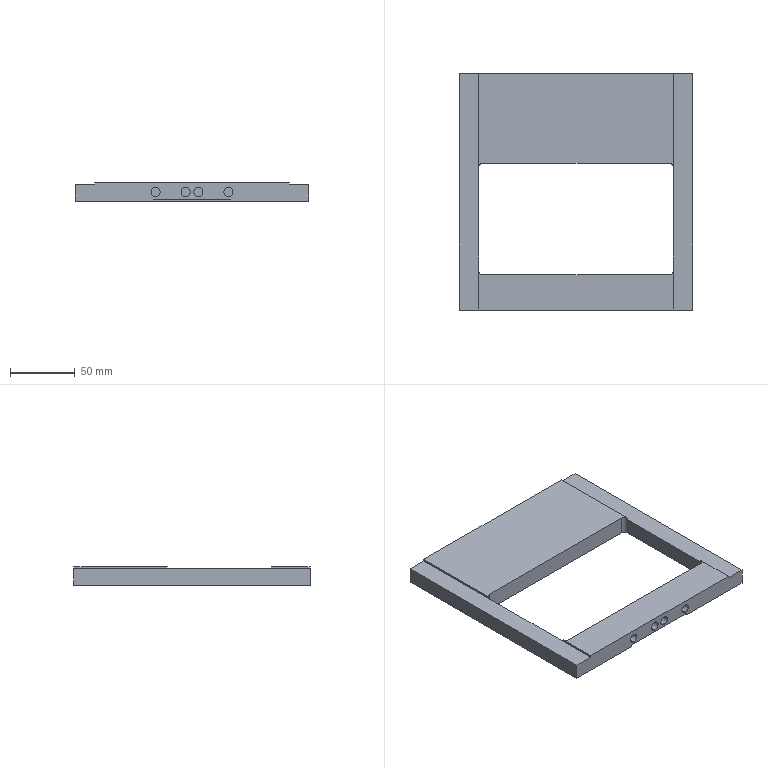Part | SolidWorks | features ICE 5, Extrusion 1, Fillet 1 | 1 solid | 47 faces | box 180 x 182 x 14 mm | volume 257706 mm3 | plane 29 | cylinder 18 | commonest cylinder face diameters 7 x8 10 x6 6 x4
STEP:
#1=CARTESIAN_POINT('',(-28.,-64.,-3.5));
#2=VERTEX_POINT('',#1);
#3=CARTESIAN_POINT('',(-28.,-64.,3.5));
#4=VERTEX_POINT('',#3);
#5=CARTESIAN_POINT('',(-28.,-64.,0.));
#6=DIRECTION('',(0.,1.,0.));
#7=DIRECTION('',(0.,0.,-1.));
#8=AXIS2_PLACEMENT_3D('',#5,#6,#7);
#9=CIRCLE('',#8,3.5);
#10=EDGE_CURVE('',#2,#4,#9,.T.);
#11=ORIENTED_EDGE('',*,*,#10,.T.);
#12=CARTESIAN_POINT('',(-28.,-91.,3.5));
#13=VERTEX_POINT('',#12);
#14=CARTESIAN_POINT('',(-28.,91.001,3.5));
#15=DIRECTION('',(0.,-1.,0.));
#16=VECTOR('',#15,1000.);
#17=LINE('',#14,#16);
#18=EDGE_CURVE('',#4,#13,#17,.T.);
#19=ORIENTED_EDGE('',*,*,#18,.T.);
#20=CARTESIAN_POINT('',(-28.,-91.,-3.5));
#21=VERTEX_POINT('',#20);
#22=CARTESIAN_POINT('',(-28.,-91.,0.));
#23=DIRECTION('',(0.,-1.,0.));
#24=DIRECTION('',(0.,0.,-1.));
#25=AXIS2_PLACEMENT_3D('',#22,#23,#24);
#26=CIRCLE('',#25,3.5);
#27=EDGE_CURVE('',#13,#21,#26,.T.);
#28=ORIENTED_EDGE('',*,*,#27,.T.);
#29=CARTESIAN_POINT('',(-28.,91.001,-3.5));
#30=DIRECTION('',(0.,-1.,0.));
#31=VECTOR('',#30,1000.);
#32=LINE('',#29,#31);
#33=EDGE_CURVE('',#2,#21,#32,.T.);
#34=ORIENTED_EDGE('',*,*,#33,.F.);
#35=EDGE_LOOP('',(#11,#19,#28,#34));
#36=FACE_OUTER_BOUND('',#35,.T.);
#37=CARTESIAN_POINT('',(-28.,91.001,0.));
#38=DIRECTION('',(0.,-1.,0.));
#39=DIRECTION('',(0.,0.,-1.));
#40=AXIS2_PLACEMENT_3D('',#37,#38,#39);
#41=CYLINDRICAL_SURFACE('',#40,3.5);
#42=ADVANCED_FACE('',(#36),#41,.F.);
#43=CARTESIAN_POINT('',(28.,-64.,-3.5));
#44=VERTEX_POINT('',#43);
#45=CARTESIAN_POINT('',(28.,-64.,3.5));
#46=VERTEX_POINT('',#45);
#47=CARTESIAN_POINT('',(28.,-64.,0.));
#48=DIRECTION('',(0.,1.,0.));
#49=DIRECTION('',(0.,0.,-1.));
#50=AXIS2_PLACEMENT_3D('',#47,#48,#49);
#51=CIRCLE('',#50,3.5);
#52=EDGE_CURVE('',#44,#46,#51,.T.);
#53=ORIENTED_EDGE('',*,*,#52,.T.);
#54=CARTESIAN_POINT('',(28.,-91.,3.5));
#55=VERTEX_POINT('',#54);
#56=CARTESIAN_POINT('',(28.,91.001,3.5));
#57=DIRECTION('',(0.,-1.,0.));
#58=VECTOR('',#57,1000.);
#59=LINE('',#56,#58);
#60=EDGE_CURVE('',#46,#55,#59,.T.);
#61=ORIENTED_EDGE('',*,*,#60,.T.);
#62=CARTESIAN_POINT('',(28.,-91.,-3.5));
#63=VERTEX_POINT('',#62);
#64=CARTESIAN_POINT('',(28.,-91.,0.));
#65=DIRECTION('',(0.,-1.,0.));
#66=DIRECTION('',(0.,0.,-1.));
#67=AXIS2_PLACEMENT_3D('',#64,#65,#66);
#68=CIRCLE('',#67,3.5);
#69=EDGE_CURVE('',#55,#63,#68,.T.);
#70=ORIENTED_EDGE('',*,*,#69,.T.);
#71=CARTESIAN_POINT('',(28.,91.001,-3.5));
#72=DIRECTION('',(0.,-1.,0.));
#73=VECTOR('',#72,1000.);
#74=LINE('',#71,#73);
#75=EDGE_CURVE('',#44,#63,#74,.T.);
#76=ORIENTED_EDGE('',*,*,#75,.F.);
#77=EDGE_LOOP('',(#53,#61,#70,#76));
#78=FACE_OUTER_BOUND('',#77,.T.);
#79=CARTESIAN_POINT('',(28.,91.001,0.));
#80=DIRECTION('',(0.,-1.,0.));
#81=DIRECTION('',(0.,0.,-1.));
#82=AXIS2_PLACEMENT_3D('',#79,#80,#81);
#83=CYLINDRICAL_SURFACE('',#82,3.5);
#84=ADVANCED_FACE('',(#78),#83,.F.);
#85=CARTESIAN_POINT('',(5.,-64.,-3.5));
#86=VERTEX_POINT('',#85);
#87=CARTESIAN_POINT('',(5.,-64.,3.5));
#88=VERTEX_POINT('',#87);
#89=CARTESIAN_POINT('',(5.,-64.,0.));
#90=DIRECTION('',(0.,1.,0.));
#91=DIRECTION('',(0.,0.,-1.));
#92=AXIS2_PLACEMENT_3D('',#89,#90,#91);
#93=CIRCLE('',#92,3.5);
#94=EDGE_CURVE('',#86,#88,#93,.T.);
#95=ORIENTED_EDGE('',*,*,#94,.T.);
#96=CARTESIAN_POINT('',(5.,-91.,3.5));
#97=VERTEX_POINT('',#96);
#98=CARTESIAN_POINT('',(5.,91.001,3.5));
#99=DIRECTION('',(0.,-1.,0.));
#100=VECTOR('',#99,1000.);
#101=LINE('',#98,#100);
#102=EDGE_CURVE('',#88,#97,#101,.T.);
#103=ORIENTED_EDGE('',*,*,#102,.T.);
#104=CARTESIAN_POINT('',(5.,-91.,-3.5));
#105=VERTEX_POINT('',#104);
#106=CARTESIAN_POINT('',(5.,-91.,0.));
#107=DIRECTION('',(0.,-1.,0.));
#108=DIRECTION('',(0.,0.,-1.));
#109=AXIS2_PLACEMENT_3D('',#106,#107,#108);
#110=CIRCLE('',#109,3.5);
#111=EDGE_CURVE('',#97,#105,#110,.T.);
#112=ORIENTED_EDGE('',*,*,#111,.T.);
#113=CARTESIAN_POINT('',(5.,91.001,-3.5));
#114=DIRECTION('',(0.,-1.,0.));
#115=VECTOR('',#114,1000.);
#116=LINE('',#113,#115);
#117=EDGE_CURVE('',#86,#105,#116,.T.);
#118=ORIENTED_EDGE('',*,*,#117,.F.);
#119=EDGE_LOOP('',(#95,#103,#112,#118));
#120=FACE_OUTER_BOUND('',#119,.T.);
#121=CARTESIAN_POINT('',(5.,91.001,0.));
#122=DIRECTION('',(0.,-1.,0.));
#123=DIRECTION('',(0.,0.,-1.));
#124=AXIS2_PLACEMENT_3D('',#121,#122,#123);
#125=CYLINDRICAL_SURFACE('',#124,3.5);
#126=ADVANCED_FACE('',(#120),#125,.F.);
#127=CARTESIAN_POINT('',(-5.,-64.,-3.5));
#128=VERTEX_POINT('',#127);
#129=CARTESIAN_POINT('',(-5.,-64.,3.5));
#130=VERTEX_POINT('',#129);
#131=CARTESIAN_POINT('',(-5.,-64.,0.));
#132=DIRECTION('',(0.,1.,0.));
#133=DIRECTION('',(0.,0.,-1.));
#134=AXIS2_PLACEMENT_3D('',#131,#132,#133);
#135=CIRCLE('',#134,3.5);
#136=EDGE_CURVE('',#128,#130,#135,.T.);
#137=ORIENTED_EDGE('',*,*,#136,.T.);
#138=CARTESIAN_POINT('',(-5.,-91.,3.5));
#139=VERTEX_POINT('',#138);
#140=CARTESIAN_POINT('',(-5.,91.001,3.5));
#141=DIRECTION('',(0.,-1.,0.));
#142=VECTOR('',#141,1000.);
#143=LINE('',#140,#142);
#144=EDGE_CURVE('',#130,#139,#143,.T.);
#145=ORIENTED_EDGE('',*,*,#144,.T.);
#146=CARTESIAN_POINT('',(-5.,-91.,-3.5));
#147=VERTEX_POINT('',#146);
#148=CARTESIAN_POINT('',(-5.,-91.,0.));
#149=DIRECTION('',(0.,-1.,0.));
#150=DIRECTION('',(0.,0.,-1.));
#151=AXIS2_PLACEMENT_3D('',#148,#149,#150);
#152=CIRCLE('',#151,3.5);
#153=EDGE_CURVE('',#139,#147,#152,.T.);
#154=ORIENTED_EDGE('',*,*,#153,.T.);
#155=CARTESIAN_POINT('',(-5.,91.001,-3.5));
#156=DIRECTION('',(0.,-1.,0.));
#157=VECTOR('',#156,1000.);
#158=LINE('',#155,#157);
#159=EDGE_CURVE('',#128,#147,#158,.T.);
#160=ORIENTED_EDGE('',*,*,#159,.F.);
#161=EDGE_LOOP('',(#137,#145,#154,#160));
#162=FACE_OUTER_BOUND('',#161,.T.);
#163=CARTESIAN_POINT('',(-5.,91.001,0.));
#164=DIRECTION('',(0.,-1.,0.));
#165=DIRECTION('',(0.,0.,-1.));
#166=AXIS2_PLACEMENT_3D('',#163,#164,#165);
#167=CYLINDRICAL_SURFACE('',#166,3.5);
#168=ADVANCED_FACE('',(#162),#167,.F.);
#169=CARTESIAN_POINT('',(-37.,-74.,-5.5));
#170=VERTEX_POINT('',#169);
#171=CARTESIAN_POINT('',(-32.,-69.,-5.5));
#172=VERTEX_POINT('',#171);
#173=CARTESIAN_POINT('',(-32.,-74.,-5.5));
#174=DIRECTION('',(0.,0.,-1.));
#175=DIRECTION('',(1.,0.,0.));
#176=AXIS2_PLACEMENT_3D('',#173,#174,#175);
#177=CIRCLE('',#176,5.);
#178=EDGE_CURVE('',#170,#172,#177,.T.);
#179=ORIENTED_EDGE('',*,*,#178,.F.);
#180=CARTESIAN_POINT('',(-37.,-74.,-7.));
#181=VERTEX_POINT('',#180);
#182=CARTESIAN_POINT('',(-37.,-74.,6.707));
#183=DIRECTION('',(0.,0.,-1.));
#184=VECTOR('',#183,1000.);
#185=LINE('',#182,#184);
#186=EDGE_CURVE('',#170,#181,#185,.T.);
#187=ORIENTED_EDGE('',*,*,#186,.T.);
#188=CARTESIAN_POINT('',(-32.,-69.,-7.));
#189=VERTEX_POINT('',#188);
#190=CARTESIAN_POINT('',(-32.,-74.,-7.));
#191=DIRECTION('',(0.,0.,-1.));
#192=DIRECTION('',(1.,0.,0.));
#193=AXIS2_PLACEMENT_3D('',#190,#191,#192);
#194=CIRCLE('',#193,5.);
#195=EDGE_CURVE('',#181,#189,#194,.T.);
#196=ORIENTED_EDGE('',*,*,#195,.T.);
#197=CARTESIAN_POINT('',(-32.,-69.,6.707));
#198=DIRECTION('',(0.,0.,-1.));
#199=VECTOR('',#198,1000.);
#200=LINE('',#197,#199);
#201=EDGE_CURVE('',#172,#189,#200,.T.);
#202=ORIENTED_EDGE('',*,*,#201,.F.);
#203=EDGE_LOOP('',(#179,#187,#196,#202));
#204=FACE_OUTER_BOUND('',#203,.T.);
#205=CARTESIAN_POINT('',(-32.,-74.,6.707));
#206=DIRECTION('',(0.,0.,-1.));
#207=DIRECTION('',(-1.,0.,0.));
#208=AXIS2_PLACEMENT_3D('',#205,#206,#207);
#209=CYLINDRICAL_SURFACE('',#208,5.);
#210=ADVANCED_FACE('',(#204),#209,.F.);
#211=CARTESIAN_POINT('',(-37.,32.,-5.5));
#212=VERTEX_POINT('',#211);
#213=CARTESIAN_POINT('',(-32.,37.,-5.5));
#214=VERTEX_POINT('',#213);
#215=CARTESIAN_POINT('',(-32.,32.,-5.5));
#216=DIRECTION('',(0.,0.,-1.));
#217=DIRECTION('',(1.,0.,0.));
#218=AXIS2_PLACEMENT_3D('',#215,#216,#217);
#219=CIRCLE('',#218,5.);
#220=EDGE_CURVE('',#212,#214,#219,.T.);
#221=ORIENTED_EDGE('',*,*,#220,.F.);
#222=CARTESIAN_POINT('',(-37.,32.,-7.));
#223=VERTEX_POINT('',#222);
#224=CARTESIAN_POINT('',(-37.,32.,6.707));
#225=DIRECTION('',(0.,0.,-1.));
#226=VECTOR('',#225,1000.);
#227=LINE('',#224,#226);
#228=EDGE_CURVE('',#212,#223,#227,.T.);
#229=ORIENTED_EDGE('',*,*,#228,.T.);
#230=CARTESIAN_POINT('',(-32.,37.,-7.));
#231=VERTEX_POINT('',#230);
#232=CARTESIAN_POINT('',(-32.,32.,-7.));
#233=DIRECTION('',(0.,0.,-1.));
#234=DIRECTION('',(-1.,0.,0.));
#235=AXIS2_PLACEMENT_3D('',#232,#233,#234);
#236=CIRCLE('',#235,5.);
#237=EDGE_CURVE('',#223,#231,#236,.T.);
#238=ORIENTED_EDGE('',*,*,#237,.T.);
#239=CARTESIAN_POINT('',(-32.,37.,6.707));
#240=DIRECTION('',(0.,0.,-1.));
#241=VECTOR('',#240,1000.);
#242=LINE('',#239,#241);
#243=EDGE_CURVE('',#214,#231,#242,.T.);
#244=ORIENTED_EDGE('',*,*,#243,.F.);
#245=EDGE_LOOP('',(#221,#229,#238,#244));
#246=FACE_OUTER_BOUND('',#245,.T.);
#247=CARTESIAN_POINT('',(-32.,32.,6.707));
#248=DIRECTION('',(0.,0.,-1.));
#249=DIRECTION('',(-1.,0.,0.));
#250=AXIS2_PLACEMENT_3D('',#247,#248,#249);
#251=CYLINDRICAL_SURFACE('',#250,5.);
#252=ADVANCED_FACE('',(#246),#251,.F.);
#253=CARTESIAN_POINT('',(-90.,91.,5.5));
#254=VERTEX_POINT('',#253);
#255=CARTESIAN_POINT('',(-90.,-91.,5.5));
#256=VERTEX_POINT('',#255);
#257=CARTESIAN_POINT('',(-90.,91.,5.5));
#258=DIRECTION('',(0.,-1.,0.));
#259=VECTOR('',#258,1000.);
#260=LINE('',#257,#259);
#261=EDGE_CURVE('',#254,#256,#260,.T.);
#262=ORIENTED_EDGE('',*,*,#261,.F.);
#263=CARTESIAN_POINT('',(-90.,91.,-7.));
#264=VERTEX_POINT('',#263);
#265=CARTESIAN_POINT('',(-90.,91.,7.));
#266=DIRECTION('',(0.,0.,-1.));
#267=VECTOR('',#266,1000.);
#268=LINE('',#265,#267);
#269=EDGE_CURVE('',#254,#264,#268,.T.);
#270=ORIENTED_EDGE('',*,*,#269,.T.);
#271=CARTESIAN_POINT('',(-90.,-91.,-7.));
#272=VERTEX_POINT('',#271);
#273=CARTESIAN_POINT('',(-90.,-91.,-7.));
#274=DIRECTION('',(0.,-1.,0.));
#275=VECTOR('',#274,1000.);
#276=LINE('',#273,#275);
#277=EDGE_CURVE('',#264,#272,#276,.T.);
#278=ORIENTED_EDGE('',*,*,#277,.T.);
#279=CARTESIAN_POINT('',(-90.,-91.,7.));
#280=DIRECTION('',(0.,0.,-1.));
#281=VECTOR('',#280,1000.);
#282=LINE('',#279,#281);
#283=EDGE_CURVE('',#256,#272,#282,.T.);
#284=ORIENTED_EDGE('',*,*,#283,.F.);
#285=EDGE_LOOP('',(#262,#270,#278,#284));
#286=FACE_OUTER_BOUND('',#285,.T.);
#287=CARTESIAN_POINT('',(-90.,-91.,7.));
#288=DIRECTION('',(1.,0.,0.));
#289=DIRECTION('',(0.,0.,-1.));
#290=AXIS2_PLACEMENT_3D('',#287,#288,#289);
#291=PLANE('',#290);
#292=ADVANCED_FACE('',(#286),#291,.F.);
#293=CARTESIAN_POINT('',(75.,91.,7.));
#294=VERTEX_POINT('',#293);
#295=CARTESIAN_POINT('',(-75.,91.,7.));
#296=VERTEX_POINT('',#295);
#297=CARTESIAN_POINT('',(-90.,91.,7.));
#298=DIRECTION('',(-1.,0.,0.));
#299=VECTOR('',#298,1000.);
#300=LINE('',#297,#299);
#301=EDGE_CURVE('',#294,#296,#300,.T.);
#302=ORIENTED_EDGE('',*,*,#301,.T.);
#303=CARTESIAN_POINT('',(-75.,19.,7.));
#304=VERTEX_POINT('',#303);
#305=CARTESIAN_POINT('',(-75.,91.,7.));
#306=DIRECTION('',(0.,1.,0.));
#307=VECTOR('',#306,1000.);
#308=LINE('',#305,#307);
#309=EDGE_CURVE('',#304,#296,#308,.T.);
#310=ORIENTED_EDGE('',*,*,#309,.F.);
#311=CARTESIAN_POINT('',(-72.,22.,7.));
#312=VERTEX_POINT('',#311);
#313=CARTESIAN_POINT('',(-72.,19.,7.));
#314=DIRECTION('',(0.,0.,-1.));
#315=DIRECTION('',(-1.,0.,0.));
#316=AXIS2_PLACEMENT_3D('',#313,#314,#315);
#317=CIRCLE('',#316,3.);
#318=EDGE_CURVE('',#304,#312,#317,.T.);
#319=ORIENTED_EDGE('',*,*,#318,.T.);
#320=CARTESIAN_POINT('',(72.,22.,7.));
#321=VERTEX_POINT('',#320);
#322=CARTESIAN_POINT('',(75.,22.,7.));
#323=DIRECTION('',(-1.,0.,0.));
#324=VECTOR('',#323,1000.);
#325=LINE('',#322,#324);
#326=EDGE_CURVE('',#321,#312,#325,.T.);
#327=ORIENTED_EDGE('',*,*,#326,.F.);
#328=CARTESIAN_POINT('',(75.,19.,7.));
#329=VERTEX_POINT('',#328);
#330=CARTESIAN_POINT('',(72.,19.,7.));
#331=DIRECTION('',(0.,0.,-1.));
#332=DIRECTION('',(-1.,0.,0.));
#333=AXIS2_PLACEMENT_3D('',#330,#331,#332);
#334=CIRCLE('',#333,3.);
#335=EDGE_CURVE('',#321,#329,#334,.T.);
#336=ORIENTED_EDGE('',*,*,#335,.T.);
#337=CARTESIAN_POINT('',(75.,91.,7.));
#338=DIRECTION('',(0.,-1.,0.));
#339=VECTOR('',#338,1000.);
#340=LINE('',#337,#339);
#341=EDGE_CURVE('',#294,#329,#340,.T.);
#342=ORIENTED_EDGE('',*,*,#341,.F.);
#343=EDGE_LOOP('',(#302,#310,#319,#327,#336,#342));
#344=FACE_OUTER_BOUND('',#343,.T.);
#345=CARTESIAN_POINT('',(0.,0.,7.));
#346=DIRECTION('',(0.,0.,-1.));
#347=DIRECTION('',(-1.,0.,0.));
#348=AXIS2_PLACEMENT_3D('',#345,#346,#347);
#349=PLANE('',#348);
#350=ADVANCED_FACE('',(#344),#349,.F.);
#351=CARTESIAN_POINT('',(-75.,-61.,5.5));
#352=VERTEX_POINT('',#351);
#353=CARTESIAN_POINT('',(-75.,19.,5.5));
#354=VERTEX_POINT('',#353);
#355=CARTESIAN_POINT('',(-75.,91.,5.5));
#356=DIRECTION('',(0.,1.,0.));
#357=VECTOR('',#356,1000.);
#358=LINE('',#355,#357);
#359=EDGE_CURVE('',#352,#354,#358,.T.);
#360=ORIENTED_EDGE('',*,*,#359,.F.);
#361=CARTESIAN_POINT('',(-75.,-61.,-7.));
#362=VERTEX_POINT('',#361);
#363=CARTESIAN_POINT('',(-75.,-61.,-7.));
#364=DIRECTION('',(0.,0.,-1.));
#365=VECTOR('',#364,1000.);
#366=LINE('',#363,#365);
#367=EDGE_CURVE('',#352,#362,#366,.T.);
#368=ORIENTED_EDGE('',*,*,#367,.T.);
#369=CARTESIAN_POINT('',(-75.,19.,-7.));
#370=VERTEX_POINT('',#369);
#371=CARTESIAN_POINT('',(-75.,-64.,-7.));
#372=DIRECTION('',(0.,1.,0.));
#373=VECTOR('',#372,1000.);
#374=LINE('',#371,#373);
#375=EDGE_CURVE('',#362,#370,#374,.T.);
#376=ORIENTED_EDGE('',*,*,#375,.T.);
#377=CARTESIAN_POINT('',(-75.,19.,7.));
#378=DIRECTION('',(0.,0.,1.));
#379=VECTOR('',#378,1000.);
#380=LINE('',#377,#379);
#381=EDGE_CURVE('',#370,#354,#380,.T.);
#382=ORIENTED_EDGE('',*,*,#381,.T.);
#383=EDGE_LOOP('',(#360,#368,#376,#382));
#384=FACE_OUTER_BOUND('',#383,.T.);
#385=CARTESIAN_POINT('',(-75.,-64.,7.001));
#386=DIRECTION('',(-1.,0.,0.));
#387=DIRECTION('',(0.,0.,1.));
#388=AXIS2_PLACEMENT_3D('',#385,#386,#387);
#389=PLANE('',#388);
#390=ADVANCED_FACE('',(#384),#389,.F.);
#391=CARTESIAN_POINT('',(90.,91.,5.5));
#392=VERTEX_POINT('',#391);
#393=CARTESIAN_POINT('',(90.,91.,-7.));
#394=VERTEX_POINT('',#393);
#395=CARTESIAN_POINT('',(90.,91.,7.));
#396=DIRECTION('',(0.,0.,-1.));
#397=VECTOR('',#396,1000.);
#398=LINE('',#395,#397);
#399=EDGE_CURVE('',#392,#394,#398,.T.);
#400=ORIENTED_EDGE('',*,*,#399,.F.);
#401=CARTESIAN_POINT('',(90.,-91.,5.5));
#402=VERTEX_POINT('',#401);
#403=CARTESIAN_POINT('',(90.,91.,5.5));
#404=DIRECTION('',(0.,1.,0.));
#405=VECTOR('',#404,1000.);
#406=LINE('',#403,#405);
#407=EDGE_CURVE('',#402,#392,#406,.T.);
#408=ORIENTED_EDGE('',*,*,#407,.F.);
#409=CARTESIAN_POINT('',(90.,-91.,-7.));
#410=VERTEX_POINT('',#409);
#411=CARTESIAN_POINT('',(90.,-91.,7.));
#412=DIRECTION('',(0.,0.,-1.));
#413=VECTOR('',#412,1000.);
#414=LINE('',#411,#413);
#415=EDGE_CURVE('',#402,#410,#414,.T.);
#416=ORIENTED_EDGE('',*,*,#415,.T.);
#417=CARTESIAN_POINT('',(90.,-91.,-7.));
#418=DIRECTION('',(0.,1.,0.));
#419=VECTOR('',#418,1000.);
#420=LINE('',#417,#419);
#421=EDGE_CURVE('',#410,#394,#420,.T.);
#422=ORIENTED_EDGE('',*,*,#421,.T.);
#423=EDGE_LOOP('',(#400,#408,#416,#422));
#424=FACE_OUTER_BOUND('',#423,.T.);
#425=CARTESIAN_POINT('',(90.,-91.,7.));
#426=DIRECTION('',(-1.,0.,0.));
#427=DIRECTION('',(0.,0.,1.));
#428=AXIS2_PLACEMENT_3D('',#425,#426,#427);
#429=PLANE('',#428);
#430=ADVANCED_FACE('',(#424),#429,.F.);
#431=CARTESIAN_POINT('',(-75.,91.,5.5));
#432=VERTEX_POINT('',#431);
#433=CARTESIAN_POINT('',(-90.,91.,5.5));
#434=DIRECTION('',(-1.,0.,0.));
#435=VECTOR('',#434,1000.);
#436=LINE('',#433,#435);
#437=EDGE_CURVE('',#432,#254,#436,.T.);
#438=ORIENTED_EDGE('',*,*,#437,.F.);
#439=CARTESIAN_POINT('',(-75.,91.,5.5));
#440=DIRECTION('',(0.,0.,1.));
#441=VECTOR('',#440,1000.);
#442=LINE('',#439,#441);
#443=EDGE_CURVE('',#432,#296,#442,.T.);
#444=ORIENTED_EDGE('',*,*,#443,.T.);
#445=ORIENTED_EDGE('',*,*,#301,.F.);
#446=CARTESIAN_POINT('',(75.,91.,5.5));
#447=VERTEX_POINT('',#446);
#448=CARTESIAN_POINT('',(75.,91.,5.5));
#449=DIRECTION('',(0.,0.,1.));
#450=VECTOR('',#449,1000.);
#451=LINE('',#448,#450);
#452=EDGE_CURVE('',#447,#294,#451,.T.);
#453=ORIENTED_EDGE('',*,*,#452,.F.);
#454=CARTESIAN_POINT('',(90.,91.,5.5));
#455=DIRECTION('',(-1.,0.,0.));
#456=VECTOR('',#455,1000.);
#457=LINE('',#454,#456);
#458=EDGE_CURVE('',#392,#447,#457,.T.);
#459=ORIENTED_EDGE('',*,*,#458,.F.);
#460=ORIENTED_EDGE('',*,*,#399,.T.);
#461=CARTESIAN_POINT('',(30.,91.,-7.));
#462=VERTEX_POINT('',#461);
#463=CARTESIAN_POINT('',(-90.,91.,-7.));
#464=DIRECTION('',(-1.,0.,0.));
#465=VECTOR('',#464,1000.);
#466=LINE('',#463,#465);
#467=EDGE_CURVE('',#394,#462,#466,.T.);
#468=ORIENTED_EDGE('',*,*,#467,.T.);
#469=CARTESIAN_POINT('',(30.,91.,-5.5));
#470=VERTEX_POINT('',#469);
#471=CARTESIAN_POINT('',(30.,91.,-5.5));
#472=DIRECTION('',(0.,0.,-1.));
#473=VECTOR('',#472,1000.);
#474=LINE('',#471,#473);
#475=EDGE_CURVE('',#470,#462,#474,.T.);
#476=ORIENTED_EDGE('',*,*,#475,.F.);
#477=CARTESIAN_POINT('',(-30.,91.,-5.5));
#478=VERTEX_POINT('',#477);
#479=CARTESIAN_POINT('',(30.,91.,-5.5));
#480=DIRECTION('',(1.,0.,0.));
#481=VECTOR('',#480,1000.);
#482=LINE('',#479,#481);
#483=EDGE_CURVE('',#478,#470,#482,.T.);
#484=ORIENTED_EDGE('',*,*,#483,.F.);
#485=CARTESIAN_POINT('',(-30.,91.,-7.));
#486=VERTEX_POINT('',#485);
#487=CARTESIAN_POINT('',(-30.,91.,-5.5));
#488=DIRECTION('',(0.,0.,-1.));
#489=VECTOR('',#488,1000.);
#490=LINE('',#487,#489);
#491=EDGE_CURVE('',#478,#486,#490,.T.);
#492=ORIENTED_EDGE('',*,*,#491,.T.);
#493=CARTESIAN_POINT('',(-90.,91.,-7.));
#494=DIRECTION('',(-1.,0.,0.));
#495=VECTOR('',#494,1000.);
#496=LINE('',#493,#495);
#497=EDGE_CURVE('',#486,#264,#496,.T.);
#498=ORIENTED_EDGE('',*,*,#497,.T.);
#499=ORIENTED_EDGE('',*,*,#269,.F.);
#500=EDGE_LOOP('',(#438,#444,#445,#453,#459,#460,#468,#476,#484,#492,#498,#499));
#501=FACE_OUTER_BOUND('',#500,.T.);
#502=CARTESIAN_POINT('',(-90.,91.,7.));
#503=DIRECTION('',(0.,-1.,0.));
#504=DIRECTION('',(0.,0.,-1.));
#505=AXIS2_PLACEMENT_3D('',#502,#503,#504);
#506=PLANE('',#505);
#507=ADVANCED_FACE('',(#501),#506,.F.);
#508=CARTESIAN_POINT('',(-28.,-91.,0.));
#509=DIRECTION('',(0.,-1.,0.));
#510=DIRECTION('',(0.,0.,-1.));
#511=AXIS2_PLACEMENT_3D('',#508,#509,#510);
#512=CIRCLE('',#511,3.5);
#513=EDGE_CURVE('',#21,#13,#512,.T.);
#514=ORIENTED_EDGE('',*,*,#513,.F.);
#515=ORIENTED_EDGE('',*,*,#27,.F.);
#516=EDGE_LOOP('',(#514,#515));
#517=FACE_BOUND('',#516,.T.);
#518=CARTESIAN_POINT('',(28.,-91.,0.));
#519=DIRECTION('',(0.,-1.,0.));
#520=DIRECTION('',(0.,0.,-1.));
#521=AXIS2_PLACEMENT_3D('',#518,#519,#520);
#522=CIRCLE('',#521,3.5);
#523=EDGE_CURVE('',#63,#55,#522,.T.);
#524=ORIENTED_EDGE('',*,*,#523,.F.);
#525=ORIENTED_EDGE('',*,*,#69,.F.);
#526=EDGE_LOOP('',(#524,#525));
#527=FACE_BOUND('',#526,.T.);
#528=CARTESIAN_POINT('',(5.,-91.,0.));
#529=DIRECTION('',(0.,-1.,0.));
#530=DIRECTION('',(0.,0.,-1.));
#531=AXIS2_PLACEMENT_3D('',#528,#529,#530);
#532=CIRCLE('',#531,3.5);
#533=EDGE_CURVE('',#105,#97,#532,.T.);
#534=ORIENTED_EDGE('',*,*,#533,.F.);
#535=ORIENTED_EDGE('',*,*,#111,.F.);
#536=EDGE_LOOP('',(#534,#535));
#537=FACE_BOUND('',#536,.T.);
#538=CARTESIAN_POINT('',(-5.,-91.,0.));
#539=DIRECTION('',(0.,-1.,0.));
#540=DIRECTION('',(0.,0.,-1.));
#541=AXIS2_PLACEMENT_3D('',#538,#539,#540);
#542=CIRCLE('',#541,3.5);
#543=EDGE_CURVE('',#147,#139,#542,.T.);
#544=ORIENTED_EDGE('',*,*,#543,.F.);
#545=ORIENTED_EDGE('',*,*,#153,.F.);
#546=EDGE_LOOP('',(#544,#545));
#547=FACE_BOUND('',#546,.T.);
#548=CARTESIAN_POINT('',(-75.,-91.,7.));
#549=VERTEX_POINT('',#548);
#550=CARTESIAN_POINT('',(75.,-91.,7.));
#551=VERTEX_POINT('',#550);
#552=CARTESIAN_POINT('',(-90.,-91.,7.));
#553=DIRECTION('',(1.,0.,0.));
#554=VECTOR('',#553,1000.);
#555=LINE('',#552,#554);
#556=EDGE_CURVE('',#549,#551,#555,.T.);
#557=ORIENTED_EDGE('',*,*,#556,.F.);
#558=CARTESIAN_POINT('',(-75.,-91.,5.5));
#559=VERTEX_POINT('',#558);
#560=CARTESIAN_POINT('',(-75.,-91.,5.5));
#561=DIRECTION('',(0.,0.,1.));
#562=VECTOR('',#561,1000.);
#563=LINE('',#560,#562);
#564=EDGE_CURVE('',#559,#549,#563,.T.);
#565=ORIENTED_EDGE('',*,*,#564,.F.);
#566=CARTESIAN_POINT('',(-90.,-91.,5.5));
#567=DIRECTION('',(1.,0.,0.));
#568=VECTOR('',#567,1000.);
#569=LINE('',#566,#568);
#570=EDGE_CURVE('',#256,#559,#569,.T.);
#571=ORIENTED_EDGE('',*,*,#570,.F.);
#572=ORIENTED_EDGE('',*,*,#283,.T.);
#573=CARTESIAN_POINT('',(-30.,-91.,-7.));
#574=VERTEX_POINT('',#573);
#575=CARTESIAN_POINT('',(-90.,-91.,-7.));
#576=DIRECTION('',(1.,0.,0.));
#577=VECTOR('',#576,1000.);
#578=LINE('',#575,#577);
#579=EDGE_CURVE('',#272,#574,#578,.T.);
#580=ORIENTED_EDGE('',*,*,#579,.T.);
#581=CARTESIAN_POINT('',(-30.,-91.,-5.5));
#582=VERTEX_POINT('',#581);
#583=CARTESIAN_POINT('',(-30.,-91.,-5.5));
#584=DIRECTION('',(0.,0.,-1.));
#585=VECTOR('',#584,1000.);
#586=LINE('',#583,#585);
#587=EDGE_CURVE('',#582,#574,#586,.T.);
#588=ORIENTED_EDGE('',*,*,#587,.F.);
#589=CARTESIAN_POINT('',(30.,-91.,-5.5));
#590=VERTEX_POINT('',#589);
#591=CARTESIAN_POINT('',(30.,-91.,-5.5));
#592=DIRECTION('',(-1.,0.,0.));
#593=VECTOR('',#592,1000.);
#594=LINE('',#591,#593);
#595=EDGE_CURVE('',#590,#582,#594,.T.);
#596=ORIENTED_EDGE('',*,*,#595,.F.);
#597=CARTESIAN_POINT('',(30.,-91.,-7.));
#598=VERTEX_POINT('',#597);
#599=CARTESIAN_POINT('',(30.,-91.,-5.5));
#600=DIRECTION('',(0.,0.,-1.));
#601=VECTOR('',#600,1000.);
#602=LINE('',#599,#601);
#603=EDGE_CURVE('',#590,#598,#602,.T.);
#604=ORIENTED_EDGE('',*,*,#603,.T.);
#605=CARTESIAN_POINT('',(-90.,-91.,-7.));
#606=DIRECTION('',(1.,0.,0.));
#607=VECTOR('',#606,1000.);
#608=LINE('',#605,#607);
#609=EDGE_CURVE('',#598,#410,#608,.T.);
#610=ORIENTED_EDGE('',*,*,#609,.T.);
#611=ORIENTED_EDGE('',*,*,#415,.F.);
#612=CARTESIAN_POINT('',(75.,-91.,5.5));
#613=VERTEX_POINT('',#612);
#614=CARTESIAN_POINT('',(90.,-91.,5.5));
#615=DIRECTION('',(1.,0.,0.));
#616=VECTOR('',#615,1000.);
#617=LINE('',#614,#616);
#618=EDGE_CURVE('',#613,#402,#617,.T.);
#619=ORIENTED_EDGE('',*,*,#618,.F.);
#620=CARTESIAN_POINT('',(75.,-91.,5.5));
#621=DIRECTION('',(0.,0.,1.));
#622=VECTOR('',#621,1000.);
#623=LINE('',#620,#622);
#624=EDGE_CURVE('',#613,#551,#623,.T.);
#625=ORIENTED_EDGE('',*,*,#624,.T.);
#626=EDGE_LOOP('',(#557,#565,#571,#572,#580,#588,#596,#604,#610,#611,#619,#625));
#627=FACE_OUTER_BOUND('',#626,.T.);
#628=CARTESIAN_POINT('',(-90.,-91.,7.));
#629=DIRECTION('',(0.,1.,0.));
#630=DIRECTION('',(0.,0.,1.));
#631=AXIS2_PLACEMENT_3D('',#628,#629,#630);
#632=PLANE('',#631);
#633=ADVANCED_FACE('',(#517,#527,#537,#547,#627),#632,.F.);
#634=CARTESIAN_POINT('',(-72.,-64.,7.));
#635=VERTEX_POINT('',#634);
#636=CARTESIAN_POINT('',(-75.,-61.,7.));
#637=VERTEX_POINT('',#636);
#638=CARTESIAN_POINT('',(-72.,-61.,7.));
#639=DIRECTION('',(0.,0.,-1.));
#640=DIRECTION('',(-1.,0.,0.));
#641=AXIS2_PLACEMENT_3D('',#638,#639,#640);
#642=CIRCLE('',#641,3.);
#643=EDGE_CURVE('',#635,#637,#642,.T.);
#644=ORIENTED_EDGE('',*,*,#643,.T.);
#645=CARTESIAN_POINT('',(-75.,91.,7.));
#646=DIRECTION('',(0.,1.,0.));
#647=VECTOR('',#646,1000.);
#648=LINE('',#645,#647);
#649=EDGE_CURVE('',#549,#637,#648,.T.);
#650=ORIENTED_EDGE('',*,*,#649,.F.);
#651=ORIENTED_EDGE('',*,*,#556,.T.);
#652=CARTESIAN_POINT('',(75.,-61.,7.));
#653=VERTEX_POINT('',#652);
#654=CARTESIAN_POINT('',(75.,91.,7.));
#655=DIRECTION('',(0.,-1.,0.));
#656=VECTOR('',#655,1000.);
#657=LINE('',#654,#656);
#658=EDGE_CURVE('',#653,#551,#657,.T.);
#659=ORIENTED_EDGE('',*,*,#658,.F.);
#660=CARTESIAN_POINT('',(72.,-64.,7.));
#661=VERTEX_POINT('',#660);
#662=CARTESIAN_POINT('',(72.,-61.,7.));
#663=DIRECTION('',(0.,0.,-1.));
#664=DIRECTION('',(-1.,0.,0.));
#665=AXIS2_PLACEMENT_3D('',#662,#663,#664);
#666=CIRCLE('',#665,3.);
#667=EDGE_CURVE('',#653,#661,#666,.T.);
#668=ORIENTED_EDGE('',*,*,#667,.T.);
#669=CARTESIAN_POINT('',(75.,-64.,7.));
#670=DIRECTION('',(1.,0.,0.));
#671=VECTOR('',#670,1000.);
#672=LINE('',#669,#671);
#673=EDGE_CURVE('',#635,#661,#672,.T.);
#674=ORIENTED_EDGE('',*,*,#673,.F.);
#675=EDGE_LOOP('',(#644,#650,#651,#659,#668,#674));
#676=FACE_OUTER_BOUND('',#675,.T.);
#677=CARTESIAN_POINT('',(0.,0.,7.));
#678=DIRECTION('',(0.,0.,-1.));
#679=DIRECTION('',(-1.,0.,0.));
#680=AXIS2_PLACEMENT_3D('',#677,#678,#679);
#681=PLANE('',#680);
#682=ADVANCED_FACE('',(#676),#681,.F.);
#683=ORIENTED_EDGE('',*,*,#375,.F.);
#684=CARTESIAN_POINT('',(-72.,-64.,-7.));
#685=VERTEX_POINT('',#684);
#686=CARTESIAN_POINT('',(-72.,-61.,-7.));
#687=DIRECTION('',(0.,0.,1.));
#688=DIRECTION('',(-1.,0.,0.));
#689=AXIS2_PLACEMENT_3D('',#686,#687,#688);
#690=CIRCLE('',#689,3.);
#691=EDGE_CURVE('',#362,#685,#690,.T.);
#692=ORIENTED_EDGE('',*,*,#691,.T.);
#693=CARTESIAN_POINT('',(72.,-64.,-7.));
#694=VERTEX_POINT('',#693);
#695=CARTESIAN_POINT('',(75.,-64.,-7.));
#696=DIRECTION('',(-1.,0.,0.));
#697=VECTOR('',#696,1000.);
#698=LINE('',#695,#697);
#699=EDGE_CURVE('',#694,#685,#698,.T.);
#700=ORIENTED_EDGE('',*,*,#699,.F.);
#701=CARTESIAN_POINT('',(75.,-61.,-7.));
#702=VERTEX_POINT('',#701);
#703=CARTESIAN_POINT('',(72.,-61.,-7.));
#704=DIRECTION('',(0.,0.,1.));
#705=DIRECTION('',(-1.,0.,0.));
#706=AXIS2_PLACEMENT_3D('',#703,#704,#705);
#707=CIRCLE('',#706,3.);
#708=EDGE_CURVE('',#694,#702,#707,.T.);
#709=ORIENTED_EDGE('',*,*,#708,.T.);
#710=CARTESIAN_POINT('',(75.,19.,-7.));
#711=VERTEX_POINT('',#710);
#712=CARTESIAN_POINT('',(75.,-64.,-7.));
#713=DIRECTION('',(0.,-1.,0.));
#714=VECTOR('',#713,1000.);
#715=LINE('',#712,#714);
#716=EDGE_CURVE('',#711,#702,#715,.T.);
#717=ORIENTED_EDGE('',*,*,#716,.F.);
#718=CARTESIAN_POINT('',(72.,22.,-7.));
#719=VERTEX_POINT('',#718);
#720=CARTESIAN_POINT('',(72.,19.,-7.));
#721=DIRECTION('',(0.,0.,1.));
#722=DIRECTION('',(-1.,0.,0.));
#723=AXIS2_PLACEMENT_3D('',#720,#721,#722);
#724=CIRCLE('',#723,3.);
#725=EDGE_CURVE('',#711,#719,#724,.T.);
#726=ORIENTED_EDGE('',*,*,#725,.T.);
#727=CARTESIAN_POINT('',(-72.,22.,-7.));
#728=VERTEX_POINT('',#727);
#729=CARTESIAN_POINT('',(75.,22.,-7.));
#730=DIRECTION('',(1.,0.,0.));
#731=VECTOR('',#730,1000.);
#732=LINE('',#729,#731);
#733=EDGE_CURVE('',#728,#719,#732,.T.);
#734=ORIENTED_EDGE('',*,*,#733,.F.);
#735=CARTESIAN_POINT('',(-72.,19.,-7.));
#736=DIRECTION('',(0.,0.,1.));
#737=DIRECTION('',(-1.,0.,0.));
#738=AXIS2_PLACEMENT_3D('',#735,#736,#737);
#739=CIRCLE('',#738,3.);
#740=EDGE_CURVE('',#728,#370,#739,.T.);
#741=ORIENTED_EDGE('',*,*,#740,.T.);
#742=EDGE_LOOP('',(#683,#692,#700,#709,#717,#726,#734,#741));
#743=FACE_BOUND('',#742,.T.);
#744=CARTESIAN_POINT('',(32.,27.,-7.));
#745=VERTEX_POINT('',#744);
#746=CARTESIAN_POINT('',(-32.,27.,-7.));
#747=VERTEX_POINT('',#746);
#748=CARTESIAN_POINT('',(30.,27.,-7.));
#749=DIRECTION('',(-1.,0.,0.));
#750=VECTOR('',#749,1000.);
#751=LINE('',#748,#750);
#752=EDGE_CURVE('',#745,#747,#751,.T.);
#753=ORIENTED_EDGE('',*,*,#752,.F.);
#754=CARTESIAN_POINT('',(32.,37.,-7.));
#755=VERTEX_POINT('',#754);
#756=CARTESIAN_POINT('',(32.,32.,-7.));
#757=DIRECTION('',(0.,0.,-1.));
#758=DIRECTION('',(1.,0.,0.));
#759=AXIS2_PLACEMENT_3D('',#756,#757,#758);
#760=CIRCLE('',#759,5.);
#761=EDGE_CURVE('',#755,#745,#760,.T.);
#762=ORIENTED_EDGE('',*,*,#761,.F.);
#763=CARTESIAN_POINT('',(30.,37.,-7.));
#764=VERTEX_POINT('',#763);
#765=CARTESIAN_POINT('',(32.,37.,-7.));
#766=DIRECTION('',(1.,0.,0.));
#767=VECTOR('',#766,1000.);
#768=LINE('',#765,#767);
#769=EDGE_CURVE('',#764,#755,#768,.T.);
#770=ORIENTED_EDGE('',*,*,#769,.F.);
#771=CARTESIAN_POINT('',(30.,27.,-7.));
#772=DIRECTION('',(0.,-1.,0.));
#773=VECTOR('',#772,1000.);
#774=LINE('',#771,#773);
#775=EDGE_CURVE('',#462,#764,#774,.T.);
#776=ORIENTED_EDGE('',*,*,#775,.F.);
#777=ORIENTED_EDGE('',*,*,#467,.F.);
#778=ORIENTED_EDGE('',*,*,#421,.F.);
#779=ORIENTED_EDGE('',*,*,#609,.F.);
#780=CARTESIAN_POINT('',(30.,-79.,-7.));
#781=VERTEX_POINT('',#780);
#782=CARTESIAN_POINT('',(30.,-91.,-7.));
#783=DIRECTION('',(0.,-1.,0.));
#784=VECTOR('',#783,1000.);
#785=LINE('',#782,#784);
#786=EDGE_CURVE('',#781,#598,#785,.T.);
#787=ORIENTED_EDGE('',*,*,#786,.F.);
#788=CARTESIAN_POINT('',(32.,-79.,-7.));
#789=VERTEX_POINT('',#788);
#790=CARTESIAN_POINT('',(32.,-79.,-7.));
#791=DIRECTION('',(-1.,0.,0.));
#792=VECTOR('',#791,1000.);
#793=LINE('',#790,#792);
#794=EDGE_CURVE('',#789,#781,#793,.T.);
#795=ORIENTED_EDGE('',*,*,#794,.F.);
#796=CARTESIAN_POINT('',(32.,-69.,-7.));
#797=VERTEX_POINT('',#796);
#798=CARTESIAN_POINT('',(32.,-74.,-7.));
#799=DIRECTION('',(0.,0.,-1.));
#800=DIRECTION('',(-1.,0.,0.));
#801=AXIS2_PLACEMENT_3D('',#798,#799,#800);
#802=CIRCLE('',#801,5.);
#803=EDGE_CURVE('',#797,#789,#802,.T.);
#804=ORIENTED_EDGE('',*,*,#803,.F.);
#805=CARTESIAN_POINT('',(30.,-69.,-7.));
#806=DIRECTION('',(1.,0.,0.));
#807=VECTOR('',#806,1000.);
#808=LINE('',#805,#807);
#809=EDGE_CURVE('',#189,#797,#808,.T.);
#810=ORIENTED_EDGE('',*,*,#809,.F.);
#811=ORIENTED_EDGE('',*,*,#195,.F.);
#812=CARTESIAN_POINT('',(-32.,-79.,-7.));
#813=VERTEX_POINT('',#812);
#814=CARTESIAN_POINT('',(-32.,-74.,-7.));
#815=DIRECTION('',(0.,0.,-1.));
#816=DIRECTION('',(1.,0.,0.));
#817=AXIS2_PLACEMENT_3D('',#814,#815,#816);
#818=CIRCLE('',#817,5.);
#819=EDGE_CURVE('',#813,#181,#818,.T.);
#820=ORIENTED_EDGE('',*,*,#819,.F.);
#821=CARTESIAN_POINT('',(-30.,-79.,-7.));
#822=VERTEX_POINT('',#821);
#823=CARTESIAN_POINT('',(-32.,-79.,-7.));
#824=DIRECTION('',(-1.,0.,0.));
#825=VECTOR('',#824,1000.);
#826=LINE('',#823,#825);
#827=EDGE_CURVE('',#822,#813,#826,.T.);
#828=ORIENTED_EDGE('',*,*,#827,.F.);
#829=CARTESIAN_POINT('',(-30.,-91.,-7.));
#830=DIRECTION('',(0.,1.,0.));
#831=VECTOR('',#830,1000.);
#832=LINE('',#829,#831);
#833=EDGE_CURVE('',#574,#822,#832,.T.);
#834=ORIENTED_EDGE('',*,*,#833,.F.);
#835=ORIENTED_EDGE('',*,*,#579,.F.);
#836=ORIENTED_EDGE('',*,*,#277,.F.);
#837=ORIENTED_EDGE('',*,*,#497,.F.);
#838=CARTESIAN_POINT('',(-30.,37.,-7.));
#839=VERTEX_POINT('',#838);
#840=CARTESIAN_POINT('',(-30.,27.,-7.));
#841=DIRECTION('',(0.,1.,0.));
#842=VECTOR('',#841,1000.);
#843=LINE('',#840,#842);
#844=EDGE_CURVE('',#839,#486,#843,.T.);
#845=ORIENTED_EDGE('',*,*,#844,.F.);
#846=CARTESIAN_POINT('',(-32.,37.,-7.));
#847=DIRECTION('',(1.,0.,0.));
#848=VECTOR('',#847,1000.);
#849=LINE('',#846,#848);
#850=EDGE_CURVE('',#231,#839,#849,.T.);
#851=ORIENTED_EDGE('',*,*,#850,.F.);
#852=ORIENTED_EDGE('',*,*,#237,.F.);
#853=CARTESIAN_POINT('',(-32.,32.,-7.));
#854=DIRECTION('',(0.,0.,-1.));
#855=DIRECTION('',(-1.,0.,0.));
#856=AXIS2_PLACEMENT_3D('',#853,#854,#855);
#857=CIRCLE('',#856,5.);
#858=EDGE_CURVE('',#747,#223,#857,.T.);
#859=ORIENTED_EDGE('',*,*,#858,.F.);
#860=EDGE_LOOP('',(#753,#762,#770,#776,#777,#778,#779,#787,#795,#804,#810,#811,#820,#828,#834,#835,#836,#837,#845,#851,#852,#859));
#861=FACE_OUTER_BOUND('',#860,.T.);
#862=CARTESIAN_POINT('',(0.,0.,-7.));
#863=DIRECTION('',(0.,0.,-1.));
#864=DIRECTION('',(-1.,0.,0.));
#865=AXIS2_PLACEMENT_3D('',#862,#863,#864);
#866=PLANE('',#865);
#867=ADVANCED_FACE('',(#743,#861),#866,.T.);
#868=ORIENTED_EDGE('',*,*,#833,.T.);
#869=CARTESIAN_POINT('',(-30.,-79.,-5.5));
#870=VERTEX_POINT('',#869);
#871=CARTESIAN_POINT('',(-30.,-79.,6.707));
#872=DIRECTION('',(0.,0.,-1.));
#873=VECTOR('',#872,1000.);
#874=LINE('',#871,#873);
#875=EDGE_CURVE('',#870,#822,#874,.T.);
#876=ORIENTED_EDGE('',*,*,#875,.F.);
#877=CARTESIAN_POINT('',(-30.,-91.,-5.5));
#878=DIRECTION('',(0.,1.,0.));
#879=VECTOR('',#878,1000.);
#880=LINE('',#877,#879);
#881=EDGE_CURVE('',#582,#870,#880,.T.);
#882=ORIENTED_EDGE('',*,*,#881,.F.);
#883=ORIENTED_EDGE('',*,*,#587,.T.);
#884=EDGE_LOOP('',(#868,#876,#882,#883));
#885=FACE_OUTER_BOUND('',#884,.T.);
#886=CARTESIAN_POINT('',(-30.,-91.,-5.5));
#887=DIRECTION('',(-1.,0.,0.));
#888=DIRECTION('',(0.,0.,1.));
#889=AXIS2_PLACEMENT_3D('',#886,#887,#888);
#890=PLANE('',#889);
#891=ADVANCED_FACE('',(#885),#890,.F.);
#892=CARTESIAN_POINT('',(30.,-79.,-5.5));
#893=VERTEX_POINT('',#892);
#894=CARTESIAN_POINT('',(30.,-91.,-5.5));
#895=DIRECTION('',(0.,-1.,0.));
#896=VECTOR('',#895,1000.);
#897=LINE('',#894,#896);
#898=EDGE_CURVE('',#893,#590,#897,.T.);
#899=ORIENTED_EDGE('',*,*,#898,.F.);
#900=CARTESIAN_POINT('',(30.,-79.,6.707));
#901=DIRECTION('',(0.,0.,-1.));
#902=VECTOR('',#901,1000.);
#903=LINE('',#900,#902);
#904=EDGE_CURVE('',#893,#781,#903,.T.);
#905=ORIENTED_EDGE('',*,*,#904,.T.);
#906=ORIENTED_EDGE('',*,*,#786,.T.);
#907=ORIENTED_EDGE('',*,*,#603,.F.);
#908=EDGE_LOOP('',(#899,#905,#906,#907));
#909=FACE_OUTER_BOUND('',#908,.T.);
#910=CARTESIAN_POINT('',(30.,-91.,-5.5));
#911=DIRECTION('',(1.,0.,0.));
#912=DIRECTION('',(0.,0.,-1.));
#913=AXIS2_PLACEMENT_3D('',#910,#911,#912);
#914=PLANE('',#913);
#915=ADVANCED_FACE('',(#909),#914,.F.);
#916=ORIENTED_EDGE('',*,*,#809,.T.);
#917=CARTESIAN_POINT('',(32.,-69.,-5.5));
#918=VERTEX_POINT('',#917);
#919=CARTESIAN_POINT('',(32.,-69.,6.707));
#920=DIRECTION('',(0.,0.,-1.));
#921=VECTOR('',#920,1000.);
#922=LINE('',#919,#921);
#923=EDGE_CURVE('',#918,#797,#922,.T.);
#924=ORIENTED_EDGE('',*,*,#923,.F.);
#925=CARTESIAN_POINT('',(30.,-69.,-5.5));
#926=DIRECTION('',(1.,0.,0.));
#927=VECTOR('',#926,1000.);
#928=LINE('',#925,#927);
#929=EDGE_CURVE('',#172,#918,#928,.T.);
#930=ORIENTED_EDGE('',*,*,#929,.F.);
#931=ORIENTED_EDGE('',*,*,#201,.T.);
#932=EDGE_LOOP('',(#916,#924,#930,#931));
#933=FACE_OUTER_BOUND('',#932,.T.);
#934=CARTESIAN_POINT('',(30.,-69.,-5.5));
#935=DIRECTION('',(0.,1.,0.));
#936=DIRECTION('',(0.,0.,1.));
#937=AXIS2_PLACEMENT_3D('',#934,#935,#936);
#938=PLANE('',#937);
#939=ADVANCED_FACE('',(#933),#938,.F.);
#940=ORIENTED_EDGE('',*,*,#881,.T.);
#941=CARTESIAN_POINT('',(-32.,-79.,-5.5));
#942=VERTEX_POINT('',#941);
#943=CARTESIAN_POINT('',(-32.,-79.,-5.5));
#944=DIRECTION('',(-1.,0.,0.));
#945=VECTOR('',#944,1000.);
#946=LINE('',#943,#945);
#947=EDGE_CURVE('',#870,#942,#946,.T.);
#948=ORIENTED_EDGE('',*,*,#947,.T.);
#949=CARTESIAN_POINT('',(-32.,-74.,-5.5));
#950=DIRECTION('',(0.,0.,-1.));
#951=DIRECTION('',(1.,0.,0.));
#952=AXIS2_PLACEMENT_3D('',#949,#950,#951);
#953=CIRCLE('',#952,5.);
#954=EDGE_CURVE('',#942,#170,#953,.T.);
#955=ORIENTED_EDGE('',*,*,#954,.T.);
#956=ORIENTED_EDGE('',*,*,#178,.T.);
#957=ORIENTED_EDGE('',*,*,#929,.T.);
#958=CARTESIAN_POINT('',(32.,-79.,-5.5));
#959=VERTEX_POINT('',#958);
#960=CARTESIAN_POINT('',(32.,-74.,-5.5));
#961=DIRECTION('',(0.,0.,-1.));
#962=DIRECTION('',(1.,0.,0.));
#963=AXIS2_PLACEMENT_3D('',#960,#961,#962);
#964=CIRCLE('',#963,5.);
#965=EDGE_CURVE('',#918,#959,#964,.T.);
#966=ORIENTED_EDGE('',*,*,#965,.T.);
#967=CARTESIAN_POINT('',(32.,-79.,-5.5));
#968=DIRECTION('',(-1.,0.,0.));
#969=VECTOR('',#968,1000.);
#970=LINE('',#967,#969);
#971=EDGE_CURVE('',#959,#893,#970,.T.);
#972=ORIENTED_EDGE('',*,*,#971,.T.);
#973=ORIENTED_EDGE('',*,*,#898,.T.);
#974=ORIENTED_EDGE('',*,*,#595,.T.);
#975=EDGE_LOOP('',(#940,#948,#955,#956,#957,#966,#972,#973,#974));
#976=FACE_OUTER_BOUND('',#975,.T.);
#977=CARTESIAN_POINT('',(0.,0.,-5.5));
#978=DIRECTION('',(0.,0.,1.));
#979=DIRECTION('',(1.,0.,0.));
#980=AXIS2_PLACEMENT_3D('',#977,#978,#979);
#981=PLANE('',#980);
#982=ADVANCED_FACE('',(#976),#981,.F.);
#983=CARTESIAN_POINT('',(-30.,37.,-5.5));
#984=VERTEX_POINT('',#983);
#985=CARTESIAN_POINT('',(-30.,27.,-5.5));
#986=DIRECTION('',(0.,1.,0.));
#987=VECTOR('',#986,1000.);
#988=LINE('',#985,#987);
#989=EDGE_CURVE('',#984,#478,#988,.T.);
#990=ORIENTED_EDGE('',*,*,#989,.F.);
#991=CARTESIAN_POINT('',(-30.,37.,6.707));
#992=DIRECTION('',(0.,0.,-1.));
#993=VECTOR('',#992,1000.);
#994=LINE('',#991,#993);
#995=EDGE_CURVE('',#984,#839,#994,.T.);
#996=ORIENTED_EDGE('',*,*,#995,.T.);
#997=ORIENTED_EDGE('',*,*,#844,.T.);
#998=ORIENTED_EDGE('',*,*,#491,.F.);
#999=EDGE_LOOP('',(#990,#996,#997,#998));
#1000=FACE_OUTER_BOUND('',#999,.T.);
#1001=CARTESIAN_POINT('',(-30.,27.,-5.5));
#1002=DIRECTION('',(-1.,0.,0.));
#1003=DIRECTION('',(0.,0.,1.));
#1004=AXIS2_PLACEMENT_3D('',#1001,#1002,#1003);
#1005=PLANE('',#1004);
#1006=ADVANCED_FACE('',(#1000),#1005,.F.);
#1007=ORIENTED_EDGE('',*,*,#752,.T.);
#1008=CARTESIAN_POINT('',(-32.,27.,-5.5));
#1009=VERTEX_POINT('',#1008);
#1010=CARTESIAN_POINT('',(-32.,27.,6.707));
#1011=DIRECTION('',(0.,0.,-1.));
#1012=VECTOR('',#1011,1000.);
#1013=LINE('',#1010,#1012);
#1014=EDGE_CURVE('',#1009,#747,#1013,.T.);
#1015=ORIENTED_EDGE('',*,*,#1014,.F.);
#1016=CARTESIAN_POINT('',(32.,27.,-5.5));
#1017=VERTEX_POINT('',#1016);
#1018=CARTESIAN_POINT('',(30.,27.,-5.5));
#1019=DIRECTION('',(-1.,0.,0.));
#1020=VECTOR('',#1019,1000.);
#1021=LINE('',#1018,#1020);
#1022=EDGE_CURVE('',#1017,#1009,#1021,.T.);
#1023=ORIENTED_EDGE('',*,*,#1022,.F.);
#1024=CARTESIAN_POINT('',(32.,27.,6.707));
#1025=DIRECTION('',(0.,0.,-1.));
#1026=VECTOR('',#1025,1000.);
#1027=LINE('',#1024,#1026);
#1028=EDGE_CURVE('',#1017,#745,#1027,.T.);
#1029=ORIENTED_EDGE('',*,*,#1028,.T.);
#1030=EDGE_LOOP('',(#1007,#1015,#1023,#1029));
#1031=FACE_OUTER_BOUND('',#1030,.T.);
#1032=CARTESIAN_POINT('',(30.,27.,-5.5));
#1033=DIRECTION('',(0.,-1.,0.));
#1034=DIRECTION('',(0.,0.,-1.));
#1035=AXIS2_PLACEMENT_3D('',#1032,#1033,#1034);
#1036=PLANE('',#1035);
#1037=ADVANCED_FACE('',(#1031),#1036,.F.);
#1038=ORIENTED_EDGE('',*,*,#775,.T.);
#1039=CARTESIAN_POINT('',(30.,37.,-5.5));
#1040=VERTEX_POINT('',#1039);
#1041=CARTESIAN_POINT('',(30.,37.,6.707));
#1042=DIRECTION('',(0.,0.,-1.));
#1043=VECTOR('',#1042,1000.);
#1044=LINE('',#1041,#1043);
#1045=EDGE_CURVE('',#1040,#764,#1044,.T.);
#1046=ORIENTED_EDGE('',*,*,#1045,.F.);
#1047=CARTESIAN_POINT('',(30.,27.,-5.5));
#1048=DIRECTION('',(0.,-1.,0.));
#1049=VECTOR('',#1048,1000.);
#1050=LINE('',#1047,#1049);
#1051=EDGE_CURVE('',#470,#1040,#1050,.T.);
#1052=ORIENTED_EDGE('',*,*,#1051,.F.);
#1053=ORIENTED_EDGE('',*,*,#475,.T.);
#1054=EDGE_LOOP('',(#1038,#1046,#1052,#1053));
#1055=FACE_OUTER_BOUND('',#1054,.T.);
#1056=CARTESIAN_POINT('',(30.,27.,-5.5));
#1057=DIRECTION('',(1.,0.,0.));
#1058=DIRECTION('',(0.,0.,-1.));
#1059=AXIS2_PLACEMENT_3D('',#1056,#1057,#1058);
#1060=PLANE('',#1059);
#1061=ADVANCED_FACE('',(#1055),#1060,.F.);
#1062=ORIENTED_EDGE('',*,*,#1022,.T.);
#1063=CARTESIAN_POINT('',(-32.,32.,-5.5));
#1064=DIRECTION('',(0.,0.,-1.));
#1065=DIRECTION('',(1.,0.,0.));
#1066=AXIS2_PLACEMENT_3D('',#1063,#1064,#1065);
#1067=CIRCLE('',#1066,5.);
#1068=EDGE_CURVE('',#1009,#212,#1067,.T.);
#1069=ORIENTED_EDGE('',*,*,#1068,.T.);
#1070=ORIENTED_EDGE('',*,*,#220,.T.);
#1071=CARTESIAN_POINT('',(-32.,37.,-5.5));
#1072=DIRECTION('',(1.,0.,0.));
#1073=VECTOR('',#1072,1000.);
#1074=LINE('',#1071,#1073);
#1075=EDGE_CURVE('',#214,#984,#1074,.T.);
#1076=ORIENTED_EDGE('',*,*,#1075,.T.);
#1077=ORIENTED_EDGE('',*,*,#989,.T.);
#1078=ORIENTED_EDGE('',*,*,#483,.T.);
#1079=ORIENTED_EDGE('',*,*,#1051,.T.);
#1080=CARTESIAN_POINT('',(32.,37.,-5.5));
#1081=VERTEX_POINT('',#1080);
#1082=CARTESIAN_POINT('',(32.,37.,-5.5));
#1083=DIRECTION('',(1.,0.,0.));
#1084=VECTOR('',#1083,1000.);
#1085=LINE('',#1082,#1084);
#1086=EDGE_CURVE('',#1040,#1081,#1085,.T.);
#1087=ORIENTED_EDGE('',*,*,#1086,.T.);
#1088=CARTESIAN_POINT('',(32.,32.,-5.5));
#1089=DIRECTION('',(0.,0.,-1.));
#1090=DIRECTION('',(1.,0.,0.));
#1091=AXIS2_PLACEMENT_3D('',#1088,#1089,#1090);
#1092=CIRCLE('',#1091,5.);
#1093=EDGE_CURVE('',#1081,#1017,#1092,.T.);
#1094=ORIENTED_EDGE('',*,*,#1093,.T.);
#1095=EDGE_LOOP('',(#1062,#1069,#1070,#1076,#1077,#1078,#1079,#1087,#1094));
#1096=FACE_OUTER_BOUND('',#1095,.T.);
#1097=CARTESIAN_POINT('',(0.,0.,-5.5));
#1098=DIRECTION('',(0.,0.,1.));
#1099=DIRECTION('',(1.,0.,0.));
#1100=AXIS2_PLACEMENT_3D('',#1097,#1098,#1099);
#1101=PLANE('',#1100);
#1102=ADVANCED_FACE('',(#1096),#1101,.F.);
#1103=ORIENTED_EDGE('',*,*,#228,.F.);
#1104=ORIENTED_EDGE('',*,*,#1068,.F.);
#1105=ORIENTED_EDGE('',*,*,#1014,.T.);
#1106=ORIENTED_EDGE('',*,*,#858,.T.);
#1107=EDGE_LOOP('',(#1103,#1104,#1105,#1106));
#1108=FACE_OUTER_BOUND('',#1107,.T.);
#1109=CARTESIAN_POINT('',(-32.,32.,6.707));
#1110=DIRECTION('',(0.,0.,-1.));
#1111=DIRECTION('',(-1.,0.,0.));
#1112=AXIS2_PLACEMENT_3D('',#1109,#1110,#1111);
#1113=CYLINDRICAL_SURFACE('',#1112,5.);
#1114=ADVANCED_FACE('',(#1108),#1113,.F.);
#1115=ORIENTED_EDGE('',*,*,#243,.T.);
#1116=ORIENTED_EDGE('',*,*,#850,.T.);
#1117=ORIENTED_EDGE('',*,*,#995,.F.);
#1118=ORIENTED_EDGE('',*,*,#1075,.F.);
#1119=EDGE_LOOP('',(#1115,#1116,#1117,#1118));
#1120=FACE_OUTER_BOUND('',#1119,.T.);
#1121=CARTESIAN_POINT('',(-32.,37.,6.707));
#1122=DIRECTION('',(0.,1.,0.));
#1123=DIRECTION('',(0.,0.,1.));
#1124=AXIS2_PLACEMENT_3D('',#1121,#1122,#1123);
#1125=PLANE('',#1124);
#1126=ADVANCED_FACE('',(#1120),#1125,.F.);
#1127=ORIENTED_EDGE('',*,*,#1045,.T.);
#1128=ORIENTED_EDGE('',*,*,#769,.T.);
#1129=CARTESIAN_POINT('',(32.,37.,6.707));
#1130=DIRECTION('',(0.,0.,-1.));
#1131=VECTOR('',#1130,1000.);
#1132=LINE('',#1129,#1131);
#1133=EDGE_CURVE('',#1081,#755,#1132,.T.);
#1134=ORIENTED_EDGE('',*,*,#1133,.F.);
#1135=ORIENTED_EDGE('',*,*,#1086,.F.);
#1136=EDGE_LOOP('',(#1127,#1128,#1134,#1135));
#1137=FACE_OUTER_BOUND('',#1136,.T.);
#1138=CARTESIAN_POINT('',(32.,37.,6.707));
#1139=DIRECTION('',(0.,1.,0.));
#1140=DIRECTION('',(0.,0.,1.));
#1141=AXIS2_PLACEMENT_3D('',#1138,#1139,#1140);
#1142=PLANE('',#1141);
#1143=ADVANCED_FACE('',(#1137),#1142,.F.);
#1144=ORIENTED_EDGE('',*,*,#1133,.T.);
#1145=ORIENTED_EDGE('',*,*,#761,.T.);
#1146=ORIENTED_EDGE('',*,*,#1028,.F.);
#1147=ORIENTED_EDGE('',*,*,#1093,.F.);
#1148=EDGE_LOOP('',(#1144,#1145,#1146,#1147));
#1149=FACE_OUTER_BOUND('',#1148,.T.);
#1150=CARTESIAN_POINT('',(32.,32.,6.707));
#1151=DIRECTION('',(0.,0.,-1.));
#1152=DIRECTION('',(-1.,0.,0.));
#1153=AXIS2_PLACEMENT_3D('',#1150,#1151,#1152);
#1154=CYLINDRICAL_SURFACE('',#1153,5.);
#1155=ADVANCED_FACE('',(#1149),#1154,.F.);
#1156=ORIENTED_EDGE('',*,*,#875,.T.);
#1157=ORIENTED_EDGE('',*,*,#827,.T.);
#1158=CARTESIAN_POINT('',(-32.,-79.,6.707));
#1159=DIRECTION('',(0.,0.,-1.));
#1160=VECTOR('',#1159,1000.);
#1161=LINE('',#1158,#1160);
#1162=EDGE_CURVE('',#942,#813,#1161,.T.);
#1163=ORIENTED_EDGE('',*,*,#1162,.F.);
#1164=ORIENTED_EDGE('',*,*,#947,.F.);
#1165=EDGE_LOOP('',(#1156,#1157,#1163,#1164));
#1166=FACE_OUTER_BOUND('',#1165,.T.);
#1167=CARTESIAN_POINT('',(-32.,-79.,6.707));
#1168=DIRECTION('',(0.,-1.,0.));
#1169=DIRECTION('',(0.,0.,-1.));
#1170=AXIS2_PLACEMENT_3D('',#1167,#1168,#1169);
#1171=PLANE('',#1170);
#1172=ADVANCED_FACE('',(#1166),#1171,.F.);
#1173=ORIENTED_EDGE('',*,*,#186,.F.);
#1174=ORIENTED_EDGE('',*,*,#954,.F.);
#1175=ORIENTED_EDGE('',*,*,#1162,.T.);
#1176=ORIENTED_EDGE('',*,*,#819,.T.);
#1177=EDGE_LOOP('',(#1173,#1174,#1175,#1176));
#1178=FACE_OUTER_BOUND('',#1177,.T.);
#1179=CARTESIAN_POINT('',(-32.,-74.,6.707));
#1180=DIRECTION('',(0.,0.,-1.));
#1181=DIRECTION('',(-1.,0.,0.));
#1182=AXIS2_PLACEMENT_3D('',#1179,#1180,#1181);
#1183=CYLINDRICAL_SURFACE('',#1182,5.);
#1184=ADVANCED_FACE('',(#1178),#1183,.F.);
#1185=CARTESIAN_POINT('',(32.,-79.,6.707));
#1186=DIRECTION('',(0.,0.,-1.));
#1187=VECTOR('',#1186,1000.);
#1188=LINE('',#1185,#1187);
#1189=EDGE_CURVE('',#959,#789,#1188,.T.);
#1190=ORIENTED_EDGE('',*,*,#1189,.T.);
#1191=ORIENTED_EDGE('',*,*,#794,.T.);
#1192=ORIENTED_EDGE('',*,*,#904,.F.);
#1193=ORIENTED_EDGE('',*,*,#971,.F.);
#1194=EDGE_LOOP('',(#1190,#1191,#1192,#1193));
#1195=FACE_OUTER_BOUND('',#1194,.T.);
#1196=CARTESIAN_POINT('',(32.,-79.,6.707));
#1197=DIRECTION('',(0.,-1.,0.));
#1198=DIRECTION('',(0.,0.,-1.));
#1199=AXIS2_PLACEMENT_3D('',#1196,#1197,#1198);
#1200=PLANE('',#1199);
#1201=ADVANCED_FACE('',(#1195),#1200,.F.);
#1202=ORIENTED_EDGE('',*,*,#923,.T.);
#1203=ORIENTED_EDGE('',*,*,#803,.T.);
#1204=ORIENTED_EDGE('',*,*,#1189,.F.);
#1205=ORIENTED_EDGE('',*,*,#965,.F.);
#1206=EDGE_LOOP('',(#1202,#1203,#1204,#1205));
#1207=FACE_OUTER_BOUND('',#1206,.T.);
#1208=CARTESIAN_POINT('',(32.,-74.,6.707));
#1209=DIRECTION('',(0.,0.,-1.));
#1210=DIRECTION('',(-1.,0.,0.));
#1211=AXIS2_PLACEMENT_3D('',#1208,#1209,#1210);
#1212=CYLINDRICAL_SURFACE('',#1211,5.);
#1213=ADVANCED_FACE('',(#1207),#1212,.F.);
#1214=ORIENTED_EDGE('',*,*,#10,.F.);
#1215=CARTESIAN_POINT('',(-28.,-64.,0.));
#1216=DIRECTION('',(0.,1.,0.));
#1217=DIRECTION('',(0.,0.,-1.));
#1218=AXIS2_PLACEMENT_3D('',#1215,#1216,#1217);
#1219=CIRCLE('',#1218,3.5);
#1220=EDGE_CURVE('',#4,#2,#1219,.T.);
#1221=ORIENTED_EDGE('',*,*,#1220,.F.);
#1222=EDGE_LOOP('',(#1214,#1221));
#1223=FACE_BOUND('',#1222,.T.);
#1224=ORIENTED_EDGE('',*,*,#52,.F.);
#1225=CARTESIAN_POINT('',(28.,-64.,0.));
#1226=DIRECTION('',(0.,1.,0.));
#1227=DIRECTION('',(0.,0.,-1.));
#1228=AXIS2_PLACEMENT_3D('',#1225,#1226,#1227);
#1229=CIRCLE('',#1228,3.5);
#1230=EDGE_CURVE('',#46,#44,#1229,.T.);
#1231=ORIENTED_EDGE('',*,*,#1230,.F.);
#1232=EDGE_LOOP('',(#1224,#1231));
#1233=FACE_BOUND('',#1232,.T.);
#1234=ORIENTED_EDGE('',*,*,#94,.F.);
#1235=CARTESIAN_POINT('',(5.,-64.,0.));
#1236=DIRECTION('',(0.,1.,0.));
#1237=DIRECTION('',(0.,0.,-1.));
#1238=AXIS2_PLACEMENT_3D('',#1235,#1236,#1237);
#1239=CIRCLE('',#1238,3.5);
#1240=EDGE_CURVE('',#88,#86,#1239,.T.);
#1241=ORIENTED_EDGE('',*,*,#1240,.F.);
#1242=EDGE_LOOP('',(#1234,#1241));
#1243=FACE_BOUND('',#1242,.T.);
#1244=ORIENTED_EDGE('',*,*,#136,.F.);
#1245=CARTESIAN_POINT('',(-5.,-64.,0.));
#1246=DIRECTION('',(0.,1.,0.));
#1247=DIRECTION('',(0.,0.,-1.));
#1248=AXIS2_PLACEMENT_3D('',#1245,#1246,#1247);
#1249=CIRCLE('',#1248,3.5);
#1250=EDGE_CURVE('',#130,#128,#1249,.T.);
#1251=ORIENTED_EDGE('',*,*,#1250,.F.);
#1252=EDGE_LOOP('',(#1244,#1251));
#1253=FACE_BOUND('',#1252,.T.);
#1254=ORIENTED_EDGE('',*,*,#673,.T.);
#1255=CARTESIAN_POINT('',(72.,-64.,-7.));
#1256=DIRECTION('',(0.,0.,-1.));
#1257=VECTOR('',#1256,1000.);
#1258=LINE('',#1255,#1257);
#1259=EDGE_CURVE('',#661,#694,#1258,.T.);
#1260=ORIENTED_EDGE('',*,*,#1259,.T.);
#1261=ORIENTED_EDGE('',*,*,#699,.T.);
#1262=CARTESIAN_POINT('',(-72.,-64.,7.));
#1263=DIRECTION('',(0.,0.,1.));
#1264=VECTOR('',#1263,1000.);
#1265=LINE('',#1262,#1264);
#1266=EDGE_CURVE('',#685,#635,#1265,.T.);
#1267=ORIENTED_EDGE('',*,*,#1266,.T.);
#1268=EDGE_LOOP('',(#1254,#1260,#1261,#1267));
#1269=FACE_OUTER_BOUND('',#1268,.T.);
#1270=CARTESIAN_POINT('',(75.,-64.,7.001));
#1271=DIRECTION('',(0.,-1.,0.));
#1272=DIRECTION('',(0.,0.,-1.));
#1273=AXIS2_PLACEMENT_3D('',#1270,#1271,#1272);
#1274=PLANE('',#1273);
#1275=ADVANCED_FACE('',(#1223,#1233,#1243,#1253,#1269),#1274,.F.);
#1276=CARTESIAN_POINT('',(75.,-61.,5.5));
#1277=VERTEX_POINT('',#1276);
#1278=CARTESIAN_POINT('',(75.,-61.,7.));
#1279=DIRECTION('',(0.,0.,1.));
#1280=VECTOR('',#1279,1000.);
#1281=LINE('',#1278,#1280);
#1282=EDGE_CURVE('',#702,#1277,#1281,.T.);
#1283=ORIENTED_EDGE('',*,*,#1282,.T.);
#1284=CARTESIAN_POINT('',(75.,19.,5.5));
#1285=VERTEX_POINT('',#1284);
#1286=CARTESIAN_POINT('',(75.,91.,5.5));
#1287=DIRECTION('',(0.,-1.,0.));
#1288=VECTOR('',#1287,1000.);
#1289=LINE('',#1286,#1288);
#1290=EDGE_CURVE('',#1285,#1277,#1289,.T.);
#1291=ORIENTED_EDGE('',*,*,#1290,.F.);
#1292=CARTESIAN_POINT('',(75.,19.,-7.));
#1293=DIRECTION('',(0.,0.,-1.));
#1294=VECTOR('',#1293,1000.);
#1295=LINE('',#1292,#1294);
#1296=EDGE_CURVE('',#1285,#711,#1295,.T.);
#1297=ORIENTED_EDGE('',*,*,#1296,.T.);
#1298=ORIENTED_EDGE('',*,*,#716,.T.);
#1299=EDGE_LOOP('',(#1283,#1291,#1297,#1298));
#1300=FACE_OUTER_BOUND('',#1299,.T.);
#1301=CARTESIAN_POINT('',(75.,-64.,7.001));
#1302=DIRECTION('',(1.,0.,0.));
#1303=DIRECTION('',(0.,0.,-1.));
#1304=AXIS2_PLACEMENT_3D('',#1301,#1302,#1303);
#1305=PLANE('',#1304);
#1306=ADVANCED_FACE('',(#1300),#1305,.F.);
#1307=ORIENTED_EDGE('',*,*,#733,.T.);
#1308=CARTESIAN_POINT('',(72.,22.,7.));
#1309=DIRECTION('',(0.,0.,1.));
#1310=VECTOR('',#1309,1000.);
#1311=LINE('',#1308,#1310);
#1312=EDGE_CURVE('',#719,#321,#1311,.T.);
#1313=ORIENTED_EDGE('',*,*,#1312,.T.);
#1314=ORIENTED_EDGE('',*,*,#326,.T.);
#1315=CARTESIAN_POINT('',(-72.,22.,-7.));
#1316=DIRECTION('',(0.,0.,-1.));
#1317=VECTOR('',#1316,1000.);
#1318=LINE('',#1315,#1317);
#1319=EDGE_CURVE('',#312,#728,#1318,.T.);
#1320=ORIENTED_EDGE('',*,*,#1319,.T.);
#1321=EDGE_LOOP('',(#1307,#1313,#1314,#1320));
#1322=FACE_OUTER_BOUND('',#1321,.T.);
#1323=CARTESIAN_POINT('',(75.,22.,7.001));
#1324=DIRECTION('',(0.,1.,0.));
#1325=DIRECTION('',(-1.,0.,0.));
#1326=AXIS2_PLACEMENT_3D('',#1323,#1324,#1325);
#1327=PLANE('',#1326);
#1328=ADVANCED_FACE('',(#1322),#1327,.F.);
#1329=ORIENTED_EDGE('',*,*,#335,.F.);
#1330=ORIENTED_EDGE('',*,*,#1312,.F.);
#1331=ORIENTED_EDGE('',*,*,#725,.F.);
#1332=ORIENTED_EDGE('',*,*,#1296,.F.);
#1333=CARTESIAN_POINT('',(75.,19.,-7.));
#1334=DIRECTION('',(0.,0.,-1.));
#1335=VECTOR('',#1334,1000.);
#1336=LINE('',#1333,#1335);
#1337=EDGE_CURVE('',#329,#1285,#1336,.T.);
#1338=ORIENTED_EDGE('',*,*,#1337,.F.);
#1339=EDGE_LOOP('',(#1329,#1330,#1331,#1332,#1338));
#1340=FACE_OUTER_BOUND('',#1339,.T.);
#1341=CARTESIAN_POINT('',(72.,19.,7.001));
#1342=DIRECTION('',(0.,0.,1.));
#1343=DIRECTION('',(1.,0.,0.));
#1344=AXIS2_PLACEMENT_3D('',#1341,#1342,#1343);
#1345=CYLINDRICAL_SURFACE('',#1344,3.);
#1346=ADVANCED_FACE('',(#1340),#1345,.F.);
#1347=ORIENTED_EDGE('',*,*,#667,.F.);
#1348=CARTESIAN_POINT('',(75.,-61.,7.));
#1349=DIRECTION('',(0.,0.,1.));
#1350=VECTOR('',#1349,1000.);
#1351=LINE('',#1348,#1350);
#1352=EDGE_CURVE('',#1277,#653,#1351,.T.);
#1353=ORIENTED_EDGE('',*,*,#1352,.F.);
#1354=ORIENTED_EDGE('',*,*,#1282,.F.);
#1355=ORIENTED_EDGE('',*,*,#708,.F.);
#1356=ORIENTED_EDGE('',*,*,#1259,.F.);
#1357=EDGE_LOOP('',(#1347,#1353,#1354,#1355,#1356));
#1358=FACE_OUTER_BOUND('',#1357,.T.);
#1359=CARTESIAN_POINT('',(72.,-61.,7.001));
#1360=DIRECTION('',(0.,0.,1.));
#1361=DIRECTION('',(1.,0.,0.));
#1362=AXIS2_PLACEMENT_3D('',#1359,#1360,#1361);
#1363=CYLINDRICAL_SURFACE('',#1362,3.);
#1364=ADVANCED_FACE('',(#1358),#1363,.F.);
#1365=ORIENTED_EDGE('',*,*,#643,.F.);
#1366=ORIENTED_EDGE('',*,*,#1266,.F.);
#1367=ORIENTED_EDGE('',*,*,#691,.F.);
#1368=ORIENTED_EDGE('',*,*,#367,.F.);
#1369=CARTESIAN_POINT('',(-75.,-61.,-7.));
#1370=DIRECTION('',(0.,0.,-1.));
#1371=VECTOR('',#1370,1000.);
#1372=LINE('',#1369,#1371);
#1373=EDGE_CURVE('',#637,#352,#1372,.T.);
#1374=ORIENTED_EDGE('',*,*,#1373,.F.);
#1375=EDGE_LOOP('',(#1365,#1366,#1367,#1368,#1374));
#1376=FACE_OUTER_BOUND('',#1375,.T.);
#1377=CARTESIAN_POINT('',(-72.,-61.,7.001));
#1378=DIRECTION('',(0.,0.,1.));
#1379=DIRECTION('',(1.,0.,0.));
#1380=AXIS2_PLACEMENT_3D('',#1377,#1378,#1379);
#1381=CYLINDRICAL_SURFACE('',#1380,3.);
#1382=ADVANCED_FACE('',(#1376),#1381,.F.);
#1383=ORIENTED_EDGE('',*,*,#318,.F.);
#1384=CARTESIAN_POINT('',(-75.,19.,7.));
#1385=DIRECTION('',(0.,0.,1.));
#1386=VECTOR('',#1385,1000.);
#1387=LINE('',#1384,#1386);
#1388=EDGE_CURVE('',#354,#304,#1387,.T.);
#1389=ORIENTED_EDGE('',*,*,#1388,.F.);
#1390=ORIENTED_EDGE('',*,*,#381,.F.);
#1391=ORIENTED_EDGE('',*,*,#740,.F.);
#1392=ORIENTED_EDGE('',*,*,#1319,.F.);
#1393=EDGE_LOOP('',(#1383,#1389,#1390,#1391,#1392));
#1394=FACE_OUTER_BOUND('',#1393,.T.);
#1395=CARTESIAN_POINT('',(-72.,19.,7.001));
#1396=DIRECTION('',(0.,0.,1.));
#1397=DIRECTION('',(1.,0.,0.));
#1398=AXIS2_PLACEMENT_3D('',#1395,#1396,#1397);
#1399=CYLINDRICAL_SURFACE('',#1398,3.);
#1400=ADVANCED_FACE('',(#1394),#1399,.F.);
#1401=ORIENTED_EDGE('',*,*,#144,.F.);
#1402=ORIENTED_EDGE('',*,*,#1250,.T.);
#1403=ORIENTED_EDGE('',*,*,#159,.T.);
#1404=ORIENTED_EDGE('',*,*,#543,.T.);
#1405=EDGE_LOOP('',(#1401,#1402,#1403,#1404));
#1406=FACE_OUTER_BOUND('',#1405,.T.);
#1407=CARTESIAN_POINT('',(-5.,91.001,0.));
#1408=DIRECTION('',(0.,-1.,0.));
#1409=DIRECTION('',(0.,0.,-1.));
#1410=AXIS2_PLACEMENT_3D('',#1407,#1408,#1409);
#1411=CYLINDRICAL_SURFACE('',#1410,3.5);
#1412=ADVANCED_FACE('',(#1406),#1411,.F.);
#1413=ORIENTED_EDGE('',*,*,#102,.F.);
#1414=ORIENTED_EDGE('',*,*,#1240,.T.);
#1415=ORIENTED_EDGE('',*,*,#117,.T.);
#1416=ORIENTED_EDGE('',*,*,#533,.T.);
#1417=EDGE_LOOP('',(#1413,#1414,#1415,#1416));
#1418=FACE_OUTER_BOUND('',#1417,.T.);
#1419=CARTESIAN_POINT('',(5.,91.001,0.));
#1420=DIRECTION('',(0.,-1.,0.));
#1421=DIRECTION('',(0.,0.,-1.));
#1422=AXIS2_PLACEMENT_3D('',#1419,#1420,#1421);
#1423=CYLINDRICAL_SURFACE('',#1422,3.5);
#1424=ADVANCED_FACE('',(#1418),#1423,.F.);
#1425=ORIENTED_EDGE('',*,*,#60,.F.);
#1426=ORIENTED_EDGE('',*,*,#1230,.T.);
#1427=ORIENTED_EDGE('',*,*,#75,.T.);
#1428=ORIENTED_EDGE('',*,*,#523,.T.);
#1429=EDGE_LOOP('',(#1425,#1426,#1427,#1428));
#1430=FACE_OUTER_BOUND('',#1429,.T.);
#1431=CARTESIAN_POINT('',(28.,91.001,0.));
#1432=DIRECTION('',(0.,-1.,0.));
#1433=DIRECTION('',(0.,0.,-1.));
#1434=AXIS2_PLACEMENT_3D('',#1431,#1432,#1433);
#1435=CYLINDRICAL_SURFACE('',#1434,3.5);
#1436=ADVANCED_FACE('',(#1430),#1435,.F.);
#1437=ORIENTED_EDGE('',*,*,#18,.F.);
#1438=ORIENTED_EDGE('',*,*,#1220,.T.);
#1439=ORIENTED_EDGE('',*,*,#33,.T.);
#1440=ORIENTED_EDGE('',*,*,#513,.T.);
#1441=EDGE_LOOP('',(#1437,#1438,#1439,#1440));
#1442=FACE_OUTER_BOUND('',#1441,.T.);
#1443=CARTESIAN_POINT('',(-28.,91.001,0.));
#1444=DIRECTION('',(0.,-1.,0.));
#1445=DIRECTION('',(0.,0.,-1.));
#1446=AXIS2_PLACEMENT_3D('',#1443,#1444,#1445);
#1447=CYLINDRICAL_SURFACE('',#1446,3.5);
#1448=ADVANCED_FACE('',(#1442),#1447,.F.);
#1449=ORIENTED_EDGE('',*,*,#309,.T.);
#1450=ORIENTED_EDGE('',*,*,#443,.F.);
#1451=CARTESIAN_POINT('',(-75.,91.,5.5));
#1452=DIRECTION('',(0.,1.,0.));
#1453=VECTOR('',#1452,1000.);
#1454=LINE('',#1451,#1453);
#1455=EDGE_CURVE('',#354,#432,#1454,.T.);
#1456=ORIENTED_EDGE('',*,*,#1455,.F.);
#1457=ORIENTED_EDGE('',*,*,#1388,.T.);
#1458=EDGE_LOOP('',(#1449,#1450,#1456,#1457));
#1459=FACE_OUTER_BOUND('',#1458,.T.);
#1460=CARTESIAN_POINT('',(-75.,91.,5.5));
#1461=DIRECTION('',(1.,0.,0.));
#1462=DIRECTION('',(0.,1.,0.));
#1463=AXIS2_PLACEMENT_3D('',#1460,#1461,#1462);
#1464=PLANE('',#1463);
#1465=ADVANCED_FACE('',(#1459),#1464,.F.);
#1466=ORIENTED_EDGE('',*,*,#1373,.T.);
#1467=CARTESIAN_POINT('',(-75.,91.,5.5));
#1468=DIRECTION('',(0.,1.,0.));
#1469=VECTOR('',#1468,1000.);
#1470=LINE('',#1467,#1469);
#1471=EDGE_CURVE('',#559,#352,#1470,.T.);
#1472=ORIENTED_EDGE('',*,*,#1471,.F.);
#1473=ORIENTED_EDGE('',*,*,#564,.T.);
#1474=ORIENTED_EDGE('',*,*,#649,.T.);
#1475=EDGE_LOOP('',(#1466,#1472,#1473,#1474));
#1476=FACE_OUTER_BOUND('',#1475,.T.);
#1477=CARTESIAN_POINT('',(-75.,91.,5.5));
#1478=DIRECTION('',(1.,0.,0.));
#1479=DIRECTION('',(0.,1.,0.));
#1480=AXIS2_PLACEMENT_3D('',#1477,#1478,#1479);
#1481=PLANE('',#1480);
#1482=ADVANCED_FACE('',(#1476),#1481,.F.);
#1483=ORIENTED_EDGE('',*,*,#261,.T.);
#1484=ORIENTED_EDGE('',*,*,#570,.T.);
#1485=ORIENTED_EDGE('',*,*,#1471,.T.);
#1486=ORIENTED_EDGE('',*,*,#359,.T.);
#1487=ORIENTED_EDGE('',*,*,#1455,.T.);
#1488=ORIENTED_EDGE('',*,*,#437,.T.);
#1489=EDGE_LOOP('',(#1483,#1484,#1485,#1486,#1487,#1488));
#1490=FACE_OUTER_BOUND('',#1489,.T.);
#1491=CARTESIAN_POINT('',(0.,0.,5.5));
#1492=DIRECTION('',(0.,0.,1.));
#1493=DIRECTION('',(1.,0.,0.));
#1494=AXIS2_PLACEMENT_3D('',#1491,#1492,#1493);
#1495=PLANE('',#1494);
#1496=ADVANCED_FACE('',(#1490),#1495,.T.);
#1497=ORIENTED_EDGE('',*,*,#658,.T.);
#1498=ORIENTED_EDGE('',*,*,#624,.F.);
#1499=CARTESIAN_POINT('',(75.,91.,5.5));
#1500=DIRECTION('',(0.,-1.,0.));
#1501=VECTOR('',#1500,1000.);
#1502=LINE('',#1499,#1501);
#1503=EDGE_CURVE('',#1277,#613,#1502,.T.);
#1504=ORIENTED_EDGE('',*,*,#1503,.F.);
#1505=ORIENTED_EDGE('',*,*,#1352,.T.);
#1506=EDGE_LOOP('',(#1497,#1498,#1504,#1505));
#1507=FACE_OUTER_BOUND('',#1506,.T.);
#1508=CARTESIAN_POINT('',(75.,91.,5.5));
#1509=DIRECTION('',(-1.,0.,0.));
#1510=DIRECTION('',(0.,-1.,0.));
#1511=AXIS2_PLACEMENT_3D('',#1508,#1509,#1510);
#1512=PLANE('',#1511);
#1513=ADVANCED_FACE('',(#1507),#1512,.F.);
#1514=ORIENTED_EDGE('',*,*,#1337,.T.);
#1515=CARTESIAN_POINT('',(75.,91.,5.5));
#1516=DIRECTION('',(0.,-1.,0.));
#1517=VECTOR('',#1516,1000.);
#1518=LINE('',#1515,#1517);
#1519=EDGE_CURVE('',#447,#1285,#1518,.T.);
#1520=ORIENTED_EDGE('',*,*,#1519,.F.);
#1521=ORIENTED_EDGE('',*,*,#452,.T.);
#1522=ORIENTED_EDGE('',*,*,#341,.T.);
#1523=EDGE_LOOP('',(#1514,#1520,#1521,#1522));
#1524=FACE_OUTER_BOUND('',#1523,.T.);
#1525=CARTESIAN_POINT('',(75.,91.,5.5));
#1526=DIRECTION('',(-1.,0.,0.));
#1527=DIRECTION('',(0.,-1.,0.));
#1528=AXIS2_PLACEMENT_3D('',#1525,#1526,#1527);
#1529=PLANE('',#1528);
#1530=ADVANCED_FACE('',(#1524),#1529,.F.);
#1531=ORIENTED_EDGE('',*,*,#407,.T.);
#1532=ORIENTED_EDGE('',*,*,#458,.T.);
#1533=ORIENTED_EDGE('',*,*,#1519,.T.);
#1534=ORIENTED_EDGE('',*,*,#1290,.T.);
#1535=ORIENTED_EDGE('',*,*,#1503,.T.);
#1536=ORIENTED_EDGE('',*,*,#618,.T.);
#1537=EDGE_LOOP('',(#1531,#1532,#1533,#1534,#1535,#1536));
#1538=FACE_OUTER_BOUND('',#1537,.T.);
#1539=CARTESIAN_POINT('',(0.,0.,5.5));
#1540=DIRECTION('',(0.,0.,-1.));
#1541=DIRECTION('',(-1.,0.,0.));
#1542=AXIS2_PLACEMENT_3D('',#1539,#1540,#1541);
#1543=PLANE('',#1542);
#1544=ADVANCED_FACE('',(#1538),#1543,.F.);
#1545=CLOSED_SHELL('',(#42,#84,#126,#168,#210,#252,#292,#350,#390,#430,#507,#633,#682,#867,#891,#915,#939,#982,#1006,#1037,#1061,#1102,#1114,#1126,#1143,#1155,#1172,#1184,#1201,#1213,#1275,#1306,#1328,#1346,#1364,#1382,#1400,#1412,#1424,#1436,#1448,#1465,#1482,#1496,#1513,#1530,#1544));
#1546=MANIFOLD_SOLID_BREP('',#1545);
#1547=CARTESIAN_POINT('',(0.,0.,0.));
#1548=DIRECTION('',(0.,0.,1.));
#1549=DIRECTION('',(1.,0.,0.));
#1550=AXIS2_PLACEMENT_3D('',#1547,#1548,#1549);
#1551=(LENGTH_UNIT()NAMED_UNIT(*)SI_UNIT(.MILLI.,.METRE.));
#1552=UNCERTAINTY_MEASURE_WITH_UNIT(LENGTH_MEASURE(0.00001),#1551,'','');
#1553=(NAMED_UNIT(*)PLANE_ANGLE_UNIT()SI_UNIT($,.RADIAN.));
#1554=(NAMED_UNIT(*)SI_UNIT($,.STERADIAN.)SOLID_ANGLE_UNIT());
#1555=(GEOMETRIC_REPRESENTATION_CONTEXT(3)GLOBAL_UNCERTAINTY_ASSIGNED_CONTEXT((#1552))GLOBAL_UNIT_ASSIGNED_CONTEXT((#1551,#1553,#1554))REPRESENTATION_CONTEXT('',''));
#1556=ADVANCED_BREP_SHAPE_REPRESENTATION('',(#1546,#1550),#1555);